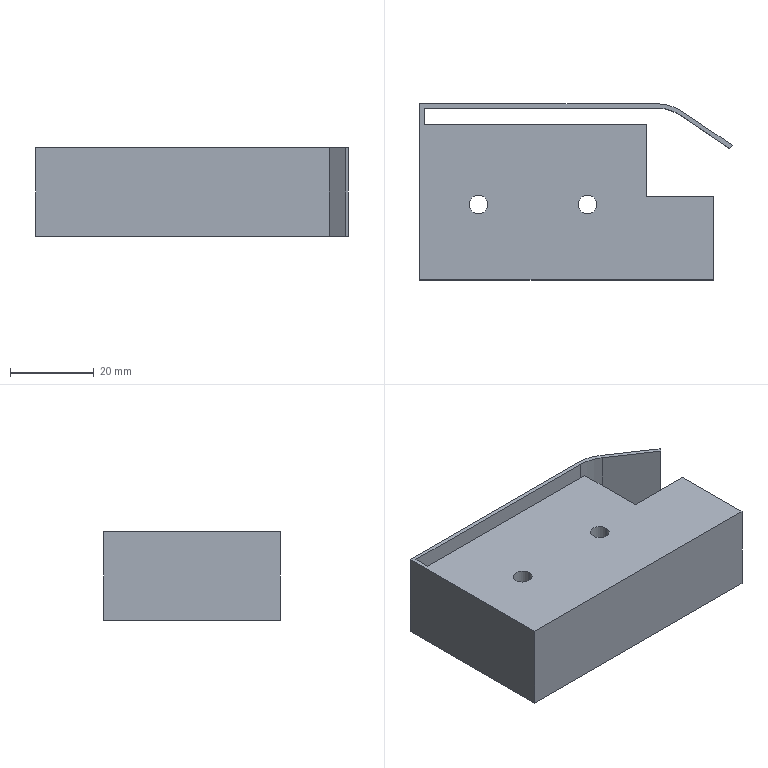Part | SolidWorks | features Extrusion 1, ICE 1 | 1 solid | 20 faces | box 74.506 x 42 x 21 mm | volume 49715 mm3 | plane 14 | cylinder 6 | commonest cylinder face diameters 4.5 x4 20 x2
STEP:
#1=CARTESIAN_POINT('',(37.75,18.,21.));
#2=VERTEX_POINT('',#1);
#3=CARTESIAN_POINT('',(42.25,18.,21.));
#4=VERTEX_POINT('',#3);
#5=CARTESIAN_POINT('',(40.,18.,21.));
#6=DIRECTION('',(0.,0.,1.));
#7=DIRECTION('',(1.,0.,0.));
#8=AXIS2_PLACEMENT_3D('',#5,#6,#7);
#9=CIRCLE('',#8,2.25);
#10=EDGE_CURVE('',#2,#4,#9,.T.);
#11=ORIENTED_EDGE('',*,*,#10,.T.);
#12=CARTESIAN_POINT('',(42.25,18.,0.));
#13=VERTEX_POINT('',#12);
#14=CARTESIAN_POINT('',(42.25,18.,21.));
#15=DIRECTION('',(0.,0.,-1.));
#16=VECTOR('',#15,1000.);
#17=LINE('',#14,#16);
#18=EDGE_CURVE('',#4,#13,#17,.T.);
#19=ORIENTED_EDGE('',*,*,#18,.T.);
#20=CARTESIAN_POINT('',(37.75,18.,0.));
#21=VERTEX_POINT('',#20);
#22=CARTESIAN_POINT('',(40.,18.,0.));
#23=DIRECTION('',(0.,0.,1.));
#24=DIRECTION('',(1.,0.,0.));
#25=AXIS2_PLACEMENT_3D('',#22,#23,#24);
#26=CIRCLE('',#25,2.25);
#27=EDGE_CURVE('',#21,#13,#26,.T.);
#28=ORIENTED_EDGE('',*,*,#27,.F.);
#29=CARTESIAN_POINT('',(37.75,18.,21.));
#30=DIRECTION('',(0.,0.,-1.));
#31=VECTOR('',#30,1000.);
#32=LINE('',#29,#31);
#33=EDGE_CURVE('',#2,#21,#32,.T.);
#34=ORIENTED_EDGE('',*,*,#33,.F.);
#35=EDGE_LOOP('',(#11,#19,#28,#34));
#36=FACE_OUTER_BOUND('',#35,.T.);
#37=CARTESIAN_POINT('',(40.,18.,21.));
#38=DIRECTION('',(0.,0.,-1.));
#39=DIRECTION('',(-1.,0.,0.));
#40=AXIS2_PLACEMENT_3D('',#37,#38,#39);
#41=CYLINDRICAL_SURFACE('',#40,2.25);
#42=ADVANCED_FACE('',(#36),#41,.F.);
#43=CARTESIAN_POINT('',(11.75,18.,21.));
#44=VERTEX_POINT('',#43);
#45=CARTESIAN_POINT('',(16.25,18.,21.));
#46=VERTEX_POINT('',#45);
#47=CARTESIAN_POINT('',(14.,18.,21.));
#48=DIRECTION('',(0.,0.,1.));
#49=DIRECTION('',(1.,0.,0.));
#50=AXIS2_PLACEMENT_3D('',#47,#48,#49);
#51=CIRCLE('',#50,2.25);
#52=EDGE_CURVE('',#44,#46,#51,.T.);
#53=ORIENTED_EDGE('',*,*,#52,.T.);
#54=CARTESIAN_POINT('',(16.25,18.,0.));
#55=VERTEX_POINT('',#54);
#56=CARTESIAN_POINT('',(16.25,18.,21.));
#57=DIRECTION('',(0.,0.,-1.));
#58=VECTOR('',#57,1000.);
#59=LINE('',#56,#58);
#60=EDGE_CURVE('',#46,#55,#59,.T.);
#61=ORIENTED_EDGE('',*,*,#60,.T.);
#62=CARTESIAN_POINT('',(11.75,18.,0.));
#63=VERTEX_POINT('',#62);
#64=CARTESIAN_POINT('',(14.,18.,0.));
#65=DIRECTION('',(0.,0.,1.));
#66=DIRECTION('',(1.,0.,0.));
#67=AXIS2_PLACEMENT_3D('',#64,#65,#66);
#68=CIRCLE('',#67,2.25);
#69=EDGE_CURVE('',#63,#55,#68,.T.);
#70=ORIENTED_EDGE('',*,*,#69,.F.);
#71=CARTESIAN_POINT('',(11.75,18.,21.));
#72=DIRECTION('',(0.,0.,-1.));
#73=VECTOR('',#72,1000.);
#74=LINE('',#71,#73);
#75=EDGE_CURVE('',#44,#63,#74,.T.);
#76=ORIENTED_EDGE('',*,*,#75,.F.);
#77=EDGE_LOOP('',(#53,#61,#70,#76));
#78=FACE_OUTER_BOUND('',#77,.T.);
#79=CARTESIAN_POINT('',(14.,18.,21.));
#80=DIRECTION('',(0.,0.,-1.));
#81=DIRECTION('',(-1.,0.,0.));
#82=AXIS2_PLACEMENT_3D('',#79,#80,#81);
#83=CYLINDRICAL_SURFACE('',#82,2.25);
#84=ADVANCED_FACE('',(#78),#83,.F.);
#85=ORIENTED_EDGE('',*,*,#52,.F.);
#86=CARTESIAN_POINT('',(14.,18.,21.));
#87=DIRECTION('',(0.,0.,1.));
#88=DIRECTION('',(1.,0.,0.));
#89=AXIS2_PLACEMENT_3D('',#86,#87,#88);
#90=CIRCLE('',#89,2.25);
#91=EDGE_CURVE('',#46,#44,#90,.T.);
#92=ORIENTED_EDGE('',*,*,#91,.F.);
#93=EDGE_LOOP('',(#85,#92));
#94=FACE_BOUND('',#93,.T.);
#95=CARTESIAN_POINT('',(0.,42.,21.));
#96=VERTEX_POINT('',#95);
#97=CARTESIAN_POINT('',(0.,0.,21.));
#98=VERTEX_POINT('',#97);
#99=CARTESIAN_POINT('',(0.,0.,21.));
#100=DIRECTION('',(0.,-1.,0.));
#101=VECTOR('',#100,1000.);
#102=LINE('',#99,#101);
#103=EDGE_CURVE('',#96,#98,#102,.T.);
#104=ORIENTED_EDGE('',*,*,#103,.T.);
#105=CARTESIAN_POINT('',(70.,0.,21.));
#106=VERTEX_POINT('',#105);
#107=CARTESIAN_POINT('',(0.,0.,21.));
#108=DIRECTION('',(1.,0.,0.));
#109=VECTOR('',#108,1000.);
#110=LINE('',#107,#109);
#111=EDGE_CURVE('',#98,#106,#110,.T.);
#112=ORIENTED_EDGE('',*,*,#111,.T.);
#113=CARTESIAN_POINT('',(70.,20.,21.));
#114=VERTEX_POINT('',#113);
#115=CARTESIAN_POINT('',(70.,0.,21.));
#116=DIRECTION('',(0.,1.,0.));
#117=VECTOR('',#116,1000.);
#118=LINE('',#115,#117);
#119=EDGE_CURVE('',#106,#114,#118,.T.);
#120=ORIENTED_EDGE('',*,*,#119,.T.);
#121=CARTESIAN_POINT('',(54.,20.,21.));
#122=VERTEX_POINT('',#121);
#123=CARTESIAN_POINT('',(54.,20.,21.));
#124=DIRECTION('',(-1.,0.,0.));
#125=VECTOR('',#124,1000.);
#126=LINE('',#123,#125);
#127=EDGE_CURVE('',#114,#122,#126,.T.);
#128=ORIENTED_EDGE('',*,*,#127,.T.);
#129=CARTESIAN_POINT('',(54.,37.,21.));
#130=VERTEX_POINT('',#129);
#131=CARTESIAN_POINT('',(54.,20.,21.));
#132=DIRECTION('',(0.,1.,0.));
#133=VECTOR('',#132,1000.);
#134=LINE('',#131,#133);
#135=EDGE_CURVE('',#122,#130,#134,.T.);
#136=ORIENTED_EDGE('',*,*,#135,.T.);
#137=CARTESIAN_POINT('',(1.,37.,21.));
#138=VERTEX_POINT('',#137);
#139=CARTESIAN_POINT('',(0.,37.,21.));
#140=DIRECTION('',(-1.,0.,0.));
#141=VECTOR('',#140,1000.);
#142=LINE('',#139,#141);
#143=EDGE_CURVE('',#130,#138,#142,.T.);
#144=ORIENTED_EDGE('',*,*,#143,.T.);
#145=CARTESIAN_POINT('',(1.,41.,21.));
#146=VERTEX_POINT('',#145);
#147=CARTESIAN_POINT('',(1.,37.,21.));
#148=DIRECTION('',(0.,1.,0.));
#149=VECTOR('',#148,1000.);
#150=LINE('',#147,#149);
#151=EDGE_CURVE('',#138,#146,#150,.T.);
#152=ORIENTED_EDGE('',*,*,#151,.T.);
#153=CARTESIAN_POINT('',(56.534,41.,21.));
#154=VERTEX_POINT('',#153);
#155=CARTESIAN_POINT('',(1.,41.,21.));
#156=DIRECTION('',(1.,0.,0.));
#157=VECTOR('',#156,1000.);
#158=LINE('',#155,#157);
#159=EDGE_CURVE('',#146,#154,#158,.T.);
#160=ORIENTED_EDGE('',*,*,#159,.T.);
#161=CARTESIAN_POINT('',(62.118,39.295,21.));
#162=VERTEX_POINT('',#161);
#163=CARTESIAN_POINT('',(56.534,31.,21.));
#164=DIRECTION('',(0.,0.,-1.));
#165=DIRECTION('',(1.,0.,0.));
#166=AXIS2_PLACEMENT_3D('',#163,#164,#165);
#167=CIRCLE('',#166,10.);
#168=EDGE_CURVE('',#154,#162,#167,.T.);
#169=ORIENTED_EDGE('',*,*,#168,.T.);
#170=CARTESIAN_POINT('',(73.948,31.331,21.));
#171=VERTEX_POINT('',#170);
#172=CARTESIAN_POINT('',(62.118,39.295,21.));
#173=DIRECTION('',(0.8295,-0.5585,0.));
#174=VECTOR('',#173,1000.);
#175=LINE('',#172,#174);
#176=EDGE_CURVE('',#162,#171,#175,.T.);
#177=ORIENTED_EDGE('',*,*,#176,.T.);
#178=CARTESIAN_POINT('',(74.506,32.16,21.));
#179=VERTEX_POINT('',#178);
#180=CARTESIAN_POINT('',(74.506,32.16,21.));
#181=DIRECTION('',(0.5585,0.8295,0.));
#182=VECTOR('',#181,1000.);
#183=LINE('',#180,#182);
#184=EDGE_CURVE('',#171,#179,#183,.T.);
#185=ORIENTED_EDGE('',*,*,#184,.T.);
#186=CARTESIAN_POINT('',(62.424,40.295,21.));
#187=VERTEX_POINT('',#186);
#188=CARTESIAN_POINT('',(62.424,40.295,21.));
#189=DIRECTION('',(-0.8295,0.5585,0.));
#190=VECTOR('',#189,1000.);
#191=LINE('',#188,#190);
#192=EDGE_CURVE('',#179,#187,#191,.T.);
#193=ORIENTED_EDGE('',*,*,#192,.T.);
#194=CARTESIAN_POINT('',(56.839,42.,21.));
#195=VERTEX_POINT('',#194);
#196=CARTESIAN_POINT('',(56.839,32.,21.));
#197=DIRECTION('',(0.,0.,1.));
#198=DIRECTION('',(1.,0.,0.));
#199=AXIS2_PLACEMENT_3D('',#196,#197,#198);
#200=CIRCLE('',#199,10.);
#201=EDGE_CURVE('',#187,#195,#200,.T.);
#202=ORIENTED_EDGE('',*,*,#201,.T.);
#203=CARTESIAN_POINT('',(0.,42.,21.));
#204=DIRECTION('',(-1.,0.,0.));
#205=VECTOR('',#204,1000.);
#206=LINE('',#203,#205);
#207=EDGE_CURVE('',#195,#96,#206,.T.);
#208=ORIENTED_EDGE('',*,*,#207,.T.);
#209=EDGE_LOOP('',(#104,#112,#120,#128,#136,#144,#152,#160,#169,#177,#185,#193,#202,#208));
#210=FACE_OUTER_BOUND('',#209,.T.);
#211=ORIENTED_EDGE('',*,*,#10,.F.);
#212=CARTESIAN_POINT('',(40.,18.,21.));
#213=DIRECTION('',(0.,0.,1.));
#214=DIRECTION('',(1.,0.,0.));
#215=AXIS2_PLACEMENT_3D('',#212,#213,#214);
#216=CIRCLE('',#215,2.25);
#217=EDGE_CURVE('',#4,#2,#216,.T.);
#218=ORIENTED_EDGE('',*,*,#217,.F.);
#219=EDGE_LOOP('',(#211,#218));
#220=FACE_BOUND('',#219,.T.);
#221=CARTESIAN_POINT('',(0.,37.,21.));
#222=DIRECTION('',(0.,0.,-1.));
#223=DIRECTION('',(-1.,0.,0.));
#224=AXIS2_PLACEMENT_3D('',#221,#222,#223);
#225=PLANE('',#224);
#226=ADVANCED_FACE('',(#94,#210,#220),#225,.F.);
#227=ORIENTED_EDGE('',*,*,#69,.T.);
#228=CARTESIAN_POINT('',(14.,18.,0.));
#229=DIRECTION('',(0.,0.,1.));
#230=DIRECTION('',(1.,0.,0.));
#231=AXIS2_PLACEMENT_3D('',#228,#229,#230);
#232=CIRCLE('',#231,2.25);
#233=EDGE_CURVE('',#55,#63,#232,.T.);
#234=ORIENTED_EDGE('',*,*,#233,.T.);
#235=EDGE_LOOP('',(#227,#234));
#236=FACE_BOUND('',#235,.T.);
#237=CARTESIAN_POINT('',(0.,42.,0.));
#238=VERTEX_POINT('',#237);
#239=CARTESIAN_POINT('',(0.,0.,0.));
#240=VERTEX_POINT('',#239);
#241=CARTESIAN_POINT('',(0.,0.,0.));
#242=DIRECTION('',(0.,-1.,0.));
#243=VECTOR('',#242,1000.);
#244=LINE('',#241,#243);
#245=EDGE_CURVE('',#238,#240,#244,.T.);
#246=ORIENTED_EDGE('',*,*,#245,.F.);
#247=CARTESIAN_POINT('',(56.839,42.,0.));
#248=VERTEX_POINT('',#247);
#249=CARTESIAN_POINT('',(0.,42.,0.));
#250=DIRECTION('',(-1.,0.,0.));
#251=VECTOR('',#250,1000.);
#252=LINE('',#249,#251);
#253=EDGE_CURVE('',#248,#238,#252,.T.);
#254=ORIENTED_EDGE('',*,*,#253,.F.);
#255=CARTESIAN_POINT('',(62.424,40.295,0.));
#256=VERTEX_POINT('',#255);
#257=CARTESIAN_POINT('',(56.839,32.,0.));
#258=DIRECTION('',(0.,0.,1.));
#259=DIRECTION('',(-1.,0.,0.));
#260=AXIS2_PLACEMENT_3D('',#257,#258,#259);
#261=CIRCLE('',#260,10.);
#262=EDGE_CURVE('',#256,#248,#261,.T.);
#263=ORIENTED_EDGE('',*,*,#262,.F.);
#264=CARTESIAN_POINT('',(74.506,32.16,0.));
#265=VERTEX_POINT('',#264);
#266=CARTESIAN_POINT('',(62.424,40.295,0.));
#267=DIRECTION('',(-0.8295,0.5585,0.));
#268=VECTOR('',#267,1000.);
#269=LINE('',#266,#268);
#270=EDGE_CURVE('',#265,#256,#269,.T.);
#271=ORIENTED_EDGE('',*,*,#270,.F.);
#272=CARTESIAN_POINT('',(73.948,31.331,0.));
#273=VERTEX_POINT('',#272);
#274=CARTESIAN_POINT('',(74.506,32.16,0.));
#275=DIRECTION('',(0.5585,0.8295,0.));
#276=VECTOR('',#275,1000.);
#277=LINE('',#274,#276);
#278=EDGE_CURVE('',#273,#265,#277,.T.);
#279=ORIENTED_EDGE('',*,*,#278,.F.);
#280=CARTESIAN_POINT('',(62.118,39.295,0.));
#281=VERTEX_POINT('',#280);
#282=CARTESIAN_POINT('',(62.118,39.295,0.));
#283=DIRECTION('',(0.8295,-0.5585,0.));
#284=VECTOR('',#283,1000.);
#285=LINE('',#282,#284);
#286=EDGE_CURVE('',#281,#273,#285,.T.);
#287=ORIENTED_EDGE('',*,*,#286,.F.);
#288=CARTESIAN_POINT('',(56.534,41.,0.));
#289=VERTEX_POINT('',#288);
#290=CARTESIAN_POINT('',(56.534,31.,0.));
#291=DIRECTION('',(0.,0.,-1.));
#292=DIRECTION('',(-1.,0.,0.));
#293=AXIS2_PLACEMENT_3D('',#290,#291,#292);
#294=CIRCLE('',#293,10.);
#295=EDGE_CURVE('',#289,#281,#294,.T.);
#296=ORIENTED_EDGE('',*,*,#295,.F.);
#297=CARTESIAN_POINT('',(1.,41.,0.));
#298=VERTEX_POINT('',#297);
#299=CARTESIAN_POINT('',(1.,41.,0.));
#300=DIRECTION('',(1.,0.,0.));
#301=VECTOR('',#300,1000.);
#302=LINE('',#299,#301);
#303=EDGE_CURVE('',#298,#289,#302,.T.);
#304=ORIENTED_EDGE('',*,*,#303,.F.);
#305=CARTESIAN_POINT('',(1.,37.,0.));
#306=VERTEX_POINT('',#305);
#307=CARTESIAN_POINT('',(1.,37.,0.));
#308=DIRECTION('',(0.,1.,0.));
#309=VECTOR('',#308,1000.);
#310=LINE('',#307,#309);
#311=EDGE_CURVE('',#306,#298,#310,.T.);
#312=ORIENTED_EDGE('',*,*,#311,.F.);
#313=CARTESIAN_POINT('',(54.,37.,0.));
#314=VERTEX_POINT('',#313);
#315=CARTESIAN_POINT('',(0.,37.,0.));
#316=DIRECTION('',(-1.,0.,0.));
#317=VECTOR('',#316,1000.);
#318=LINE('',#315,#317);
#319=EDGE_CURVE('',#314,#306,#318,.T.);
#320=ORIENTED_EDGE('',*,*,#319,.F.);
#321=CARTESIAN_POINT('',(54.,20.,0.));
#322=VERTEX_POINT('',#321);
#323=CARTESIAN_POINT('',(54.,20.,0.));
#324=DIRECTION('',(0.,1.,0.));
#325=VECTOR('',#324,1000.);
#326=LINE('',#323,#325);
#327=EDGE_CURVE('',#322,#314,#326,.T.);
#328=ORIENTED_EDGE('',*,*,#327,.F.);
#329=CARTESIAN_POINT('',(70.,20.,0.));
#330=VERTEX_POINT('',#329);
#331=CARTESIAN_POINT('',(54.,20.,0.));
#332=DIRECTION('',(-1.,0.,0.));
#333=VECTOR('',#332,1000.);
#334=LINE('',#331,#333);
#335=EDGE_CURVE('',#330,#322,#334,.T.);
#336=ORIENTED_EDGE('',*,*,#335,.F.);
#337=CARTESIAN_POINT('',(70.,0.,0.));
#338=VERTEX_POINT('',#337);
#339=CARTESIAN_POINT('',(70.,0.,0.));
#340=DIRECTION('',(0.,1.,0.));
#341=VECTOR('',#340,1000.);
#342=LINE('',#339,#341);
#343=EDGE_CURVE('',#338,#330,#342,.T.);
#344=ORIENTED_EDGE('',*,*,#343,.F.);
#345=CARTESIAN_POINT('',(0.,0.,0.));
#346=DIRECTION('',(1.,0.,0.));
#347=VECTOR('',#346,1000.);
#348=LINE('',#345,#347);
#349=EDGE_CURVE('',#240,#338,#348,.T.);
#350=ORIENTED_EDGE('',*,*,#349,.F.);
#351=EDGE_LOOP('',(#246,#254,#263,#271,#279,#287,#296,#304,#312,#320,#328,#336,#344,#350));
#352=FACE_OUTER_BOUND('',#351,.T.);
#353=ORIENTED_EDGE('',*,*,#27,.T.);
#354=CARTESIAN_POINT('',(40.,18.,0.));
#355=DIRECTION('',(0.,0.,1.));
#356=DIRECTION('',(1.,0.,0.));
#357=AXIS2_PLACEMENT_3D('',#354,#355,#356);
#358=CIRCLE('',#357,2.25);
#359=EDGE_CURVE('',#13,#21,#358,.T.);
#360=ORIENTED_EDGE('',*,*,#359,.T.);
#361=EDGE_LOOP('',(#353,#360));
#362=FACE_BOUND('',#361,.T.);
#363=CARTESIAN_POINT('',(0.,37.,0.));
#364=DIRECTION('',(0.,0.,-1.));
#365=DIRECTION('',(-1.,0.,0.));
#366=AXIS2_PLACEMENT_3D('',#363,#364,#365);
#367=PLANE('',#366);
#368=ADVANCED_FACE('',(#236,#352,#362),#367,.T.);
#369=ORIENTED_EDGE('',*,*,#245,.T.);
#370=CARTESIAN_POINT('',(0.,0.,21.));
#371=DIRECTION('',(0.,0.,-1.));
#372=VECTOR('',#371,1000.);
#373=LINE('',#370,#372);
#374=EDGE_CURVE('',#98,#240,#373,.T.);
#375=ORIENTED_EDGE('',*,*,#374,.F.);
#376=ORIENTED_EDGE('',*,*,#103,.F.);
#377=CARTESIAN_POINT('',(0.,42.,-75.266));
#378=DIRECTION('',(0.,0.,1.));
#379=VECTOR('',#378,1000.);
#380=LINE('',#377,#379);
#381=EDGE_CURVE('',#238,#96,#380,.T.);
#382=ORIENTED_EDGE('',*,*,#381,.F.);
#383=EDGE_LOOP('',(#369,#375,#376,#382));
#384=FACE_OUTER_BOUND('',#383,.T.);
#385=CARTESIAN_POINT('',(0.,0.,21.));
#386=DIRECTION('',(1.,0.,0.));
#387=DIRECTION('',(0.,0.,-1.));
#388=AXIS2_PLACEMENT_3D('',#385,#386,#387);
#389=PLANE('',#388);
#390=ADVANCED_FACE('',(#384),#389,.F.);
#391=ORIENTED_EDGE('',*,*,#349,.T.);
#392=CARTESIAN_POINT('',(70.,0.,21.));
#393=DIRECTION('',(0.,0.,-1.));
#394=VECTOR('',#393,1000.);
#395=LINE('',#392,#394);
#396=EDGE_CURVE('',#106,#338,#395,.T.);
#397=ORIENTED_EDGE('',*,*,#396,.F.);
#398=ORIENTED_EDGE('',*,*,#111,.F.);
#399=ORIENTED_EDGE('',*,*,#374,.T.);
#400=EDGE_LOOP('',(#391,#397,#398,#399));
#401=FACE_OUTER_BOUND('',#400,.T.);
#402=CARTESIAN_POINT('',(0.,0.,21.));
#403=DIRECTION('',(0.,1.,0.));
#404=DIRECTION('',(0.,0.,1.));
#405=AXIS2_PLACEMENT_3D('',#402,#403,#404);
#406=PLANE('',#405);
#407=ADVANCED_FACE('',(#401),#406,.F.);
#408=ORIENTED_EDGE('',*,*,#343,.T.);
#409=CARTESIAN_POINT('',(70.,20.,21.));
#410=DIRECTION('',(0.,0.,-1.));
#411=VECTOR('',#410,1000.);
#412=LINE('',#409,#411);
#413=EDGE_CURVE('',#114,#330,#412,.T.);
#414=ORIENTED_EDGE('',*,*,#413,.F.);
#415=ORIENTED_EDGE('',*,*,#119,.F.);
#416=ORIENTED_EDGE('',*,*,#396,.T.);
#417=EDGE_LOOP('',(#408,#414,#415,#416));
#418=FACE_OUTER_BOUND('',#417,.T.);
#419=CARTESIAN_POINT('',(70.,0.,21.));
#420=DIRECTION('',(-1.,0.,0.));
#421=DIRECTION('',(0.,0.,1.));
#422=AXIS2_PLACEMENT_3D('',#419,#420,#421);
#423=PLANE('',#422);
#424=ADVANCED_FACE('',(#418),#423,.F.);
#425=ORIENTED_EDGE('',*,*,#335,.T.);
#426=CARTESIAN_POINT('',(54.,20.,21.));
#427=DIRECTION('',(0.,0.,-1.));
#428=VECTOR('',#427,1000.);
#429=LINE('',#426,#428);
#430=EDGE_CURVE('',#122,#322,#429,.T.);
#431=ORIENTED_EDGE('',*,*,#430,.F.);
#432=ORIENTED_EDGE('',*,*,#127,.F.);
#433=ORIENTED_EDGE('',*,*,#413,.T.);
#434=EDGE_LOOP('',(#425,#431,#432,#433));
#435=FACE_OUTER_BOUND('',#434,.T.);
#436=CARTESIAN_POINT('',(54.,20.,21.));
#437=DIRECTION('',(0.,-1.,0.));
#438=DIRECTION('',(0.,0.,-1.));
#439=AXIS2_PLACEMENT_3D('',#436,#437,#438);
#440=PLANE('',#439);
#441=ADVANCED_FACE('',(#435),#440,.F.);
#442=ORIENTED_EDGE('',*,*,#327,.T.);
#443=CARTESIAN_POINT('',(54.,37.,21.));
#444=DIRECTION('',(0.,0.,-1.));
#445=VECTOR('',#444,1000.);
#446=LINE('',#443,#445);
#447=EDGE_CURVE('',#130,#314,#446,.T.);
#448=ORIENTED_EDGE('',*,*,#447,.F.);
#449=ORIENTED_EDGE('',*,*,#135,.F.);
#450=ORIENTED_EDGE('',*,*,#430,.T.);
#451=EDGE_LOOP('',(#442,#448,#449,#450));
#452=FACE_OUTER_BOUND('',#451,.T.);
#453=CARTESIAN_POINT('',(54.,20.,21.));
#454=DIRECTION('',(-1.,0.,0.));
#455=DIRECTION('',(0.,0.,1.));
#456=AXIS2_PLACEMENT_3D('',#453,#454,#455);
#457=PLANE('',#456);
#458=ADVANCED_FACE('',(#452),#457,.F.);
#459=ORIENTED_EDGE('',*,*,#319,.T.);
#460=CARTESIAN_POINT('',(1.,37.,-75.266));
#461=DIRECTION('',(0.,0.,1.));
#462=VECTOR('',#461,1000.);
#463=LINE('',#460,#462);
#464=EDGE_CURVE('',#306,#138,#463,.T.);
#465=ORIENTED_EDGE('',*,*,#464,.T.);
#466=ORIENTED_EDGE('',*,*,#143,.F.);
#467=ORIENTED_EDGE('',*,*,#447,.T.);
#468=EDGE_LOOP('',(#459,#465,#466,#467));
#469=FACE_OUTER_BOUND('',#468,.T.);
#470=CARTESIAN_POINT('',(0.,37.,21.));
#471=DIRECTION('',(0.,-1.,0.));
#472=DIRECTION('',(0.,0.,-1.));
#473=AXIS2_PLACEMENT_3D('',#470,#471,#472);
#474=PLANE('',#473);
#475=ADVANCED_FACE('',(#469),#474,.F.);
#476=ORIENTED_EDGE('',*,*,#60,.F.);
#477=ORIENTED_EDGE('',*,*,#91,.T.);
#478=ORIENTED_EDGE('',*,*,#75,.T.);
#479=ORIENTED_EDGE('',*,*,#233,.F.);
#480=EDGE_LOOP('',(#476,#477,#478,#479));
#481=FACE_OUTER_BOUND('',#480,.T.);
#482=CARTESIAN_POINT('',(14.,18.,21.));
#483=DIRECTION('',(0.,0.,-1.));
#484=DIRECTION('',(-1.,0.,0.));
#485=AXIS2_PLACEMENT_3D('',#482,#483,#484);
#486=CYLINDRICAL_SURFACE('',#485,2.25);
#487=ADVANCED_FACE('',(#481),#486,.F.);
#488=ORIENTED_EDGE('',*,*,#18,.F.);
#489=ORIENTED_EDGE('',*,*,#217,.T.);
#490=ORIENTED_EDGE('',*,*,#33,.T.);
#491=ORIENTED_EDGE('',*,*,#359,.F.);
#492=EDGE_LOOP('',(#488,#489,#490,#491));
#493=FACE_OUTER_BOUND('',#492,.T.);
#494=CARTESIAN_POINT('',(40.,18.,21.));
#495=DIRECTION('',(0.,0.,-1.));
#496=DIRECTION('',(-1.,0.,0.));
#497=AXIS2_PLACEMENT_3D('',#494,#495,#496);
#498=CYLINDRICAL_SURFACE('',#497,2.25);
#499=ADVANCED_FACE('',(#493),#498,.F.);
#500=ORIENTED_EDGE('',*,*,#464,.F.);
#501=ORIENTED_EDGE('',*,*,#311,.T.);
#502=CARTESIAN_POINT('',(1.,41.,-75.266));
#503=DIRECTION('',(0.,0.,1.));
#504=VECTOR('',#503,1000.);
#505=LINE('',#502,#504);
#506=EDGE_CURVE('',#298,#146,#505,.T.);
#507=ORIENTED_EDGE('',*,*,#506,.T.);
#508=ORIENTED_EDGE('',*,*,#151,.F.);
#509=EDGE_LOOP('',(#500,#501,#507,#508));
#510=FACE_OUTER_BOUND('',#509,.T.);
#511=CARTESIAN_POINT('',(1.,37.,-75.266));
#512=DIRECTION('',(1.,0.,0.));
#513=DIRECTION('',(0.,0.,-1.));
#514=AXIS2_PLACEMENT_3D('',#511,#512,#513);
#515=PLANE('',#514);
#516=ADVANCED_FACE('',(#510),#515,.T.);
#517=ORIENTED_EDGE('',*,*,#506,.F.);
#518=ORIENTED_EDGE('',*,*,#303,.T.);
#519=CARTESIAN_POINT('',(56.534,41.,-75.266));
#520=DIRECTION('',(0.,0.,1.));
#521=VECTOR('',#520,1000.);
#522=LINE('',#519,#521);
#523=EDGE_CURVE('',#289,#154,#522,.T.);
#524=ORIENTED_EDGE('',*,*,#523,.T.);
#525=ORIENTED_EDGE('',*,*,#159,.F.);
#526=EDGE_LOOP('',(#517,#518,#524,#525));
#527=FACE_OUTER_BOUND('',#526,.T.);
#528=CARTESIAN_POINT('',(1.,41.,-75.266));
#529=DIRECTION('',(0.,-1.,0.));
#530=DIRECTION('',(0.,0.,-1.));
#531=AXIS2_PLACEMENT_3D('',#528,#529,#530);
#532=PLANE('',#531);
#533=ADVANCED_FACE('',(#527),#532,.T.);
#534=ORIENTED_EDGE('',*,*,#523,.F.);
#535=ORIENTED_EDGE('',*,*,#295,.T.);
#536=CARTESIAN_POINT('',(62.118,39.295,-75.266));
#537=DIRECTION('',(0.,0.,1.));
#538=VECTOR('',#537,1000.);
#539=LINE('',#536,#538);
#540=EDGE_CURVE('',#281,#162,#539,.T.);
#541=ORIENTED_EDGE('',*,*,#540,.T.);
#542=ORIENTED_EDGE('',*,*,#168,.F.);
#543=EDGE_LOOP('',(#534,#535,#541,#542));
#544=FACE_OUTER_BOUND('',#543,.T.);
#545=CARTESIAN_POINT('',(56.534,31.,-75.266));
#546=DIRECTION('',(0.,0.,1.));
#547=DIRECTION('',(1.,0.,0.));
#548=AXIS2_PLACEMENT_3D('',#545,#546,#547);
#549=CYLINDRICAL_SURFACE('',#548,10.);
#550=ADVANCED_FACE('',(#544),#549,.F.);
#551=ORIENTED_EDGE('',*,*,#540,.F.);
#552=ORIENTED_EDGE('',*,*,#286,.T.);
#553=CARTESIAN_POINT('',(73.948,31.331,-75.266));
#554=DIRECTION('',(0.,0.,1.));
#555=VECTOR('',#554,1000.);
#556=LINE('',#553,#555);
#557=EDGE_CURVE('',#273,#171,#556,.T.);
#558=ORIENTED_EDGE('',*,*,#557,.T.);
#559=ORIENTED_EDGE('',*,*,#176,.F.);
#560=EDGE_LOOP('',(#551,#552,#558,#559));
#561=FACE_OUTER_BOUND('',#560,.T.);
#562=CARTESIAN_POINT('',(62.118,39.295,-75.266));
#563=DIRECTION('',(-0.5585,-0.8295,0.));
#564=DIRECTION('',(0.8295,-0.5585,0.));
#565=AXIS2_PLACEMENT_3D('',#562,#563,#564);
#566=PLANE('',#565);
#567=ADVANCED_FACE('',(#561),#566,.T.);
#568=ORIENTED_EDGE('',*,*,#557,.F.);
#569=ORIENTED_EDGE('',*,*,#278,.T.);
#570=CARTESIAN_POINT('',(74.506,32.16,-75.266));
#571=DIRECTION('',(0.,0.,1.));
#572=VECTOR('',#571,1000.);
#573=LINE('',#570,#572);
#574=EDGE_CURVE('',#265,#179,#573,.T.);
#575=ORIENTED_EDGE('',*,*,#574,.T.);
#576=ORIENTED_EDGE('',*,*,#184,.F.);
#577=EDGE_LOOP('',(#568,#569,#575,#576));
#578=FACE_OUTER_BOUND('',#577,.T.);
#579=CARTESIAN_POINT('',(74.506,32.16,-75.266));
#580=DIRECTION('',(0.8295,-0.5585,0.));
#581=DIRECTION('',(0.5585,0.8295,0.));
#582=AXIS2_PLACEMENT_3D('',#579,#580,#581);
#583=PLANE('',#582);
#584=ADVANCED_FACE('',(#578),#583,.T.);
#585=ORIENTED_EDGE('',*,*,#574,.F.);
#586=ORIENTED_EDGE('',*,*,#270,.T.);
#587=CARTESIAN_POINT('',(62.424,40.295,-75.266));
#588=DIRECTION('',(0.,0.,1.));
#589=VECTOR('',#588,1000.);
#590=LINE('',#587,#589);
#591=EDGE_CURVE('',#256,#187,#590,.T.);
#592=ORIENTED_EDGE('',*,*,#591,.T.);
#593=ORIENTED_EDGE('',*,*,#192,.F.);
#594=EDGE_LOOP('',(#585,#586,#592,#593));
#595=FACE_OUTER_BOUND('',#594,.T.);
#596=CARTESIAN_POINT('',(62.424,40.295,-75.266));
#597=DIRECTION('',(0.5585,0.8295,0.));
#598=DIRECTION('',(-0.8295,0.5585,0.));
#599=AXIS2_PLACEMENT_3D('',#596,#597,#598);
#600=PLANE('',#599);
#601=ADVANCED_FACE('',(#595),#600,.T.);
#602=ORIENTED_EDGE('',*,*,#591,.F.);
#603=ORIENTED_EDGE('',*,*,#262,.T.);
#604=CARTESIAN_POINT('',(56.839,42.,-75.266));
#605=DIRECTION('',(0.,0.,1.));
#606=VECTOR('',#605,1000.);
#607=LINE('',#604,#606);
#608=EDGE_CURVE('',#248,#195,#607,.T.);
#609=ORIENTED_EDGE('',*,*,#608,.T.);
#610=ORIENTED_EDGE('',*,*,#201,.F.);
#611=EDGE_LOOP('',(#602,#603,#609,#610));
#612=FACE_OUTER_BOUND('',#611,.T.);
#613=CARTESIAN_POINT('',(56.839,32.,-75.266));
#614=DIRECTION('',(0.,0.,1.));
#615=DIRECTION('',(1.,0.,0.));
#616=AXIS2_PLACEMENT_3D('',#613,#614,#615);
#617=CYLINDRICAL_SURFACE('',#616,10.);
#618=ADVANCED_FACE('',(#612),#617,.T.);
#619=ORIENTED_EDGE('',*,*,#608,.F.);
#620=ORIENTED_EDGE('',*,*,#253,.T.);
#621=ORIENTED_EDGE('',*,*,#381,.T.);
#622=ORIENTED_EDGE('',*,*,#207,.F.);
#623=EDGE_LOOP('',(#619,#620,#621,#622));
#624=FACE_OUTER_BOUND('',#623,.T.);
#625=CARTESIAN_POINT('',(0.,42.,-75.266));
#626=DIRECTION('',(0.,1.,0.));
#627=DIRECTION('',(0.,0.,1.));
#628=AXIS2_PLACEMENT_3D('',#625,#626,#627);
#629=PLANE('',#628);
#630=ADVANCED_FACE('',(#624),#629,.T.);
#631=CLOSED_SHELL('',(#42,#84,#226,#368,#390,#407,#424,#441,#458,#475,#487,#499,#516,#533,#550,#567,#584,#601,#618,#630));
#632=MANIFOLD_SOLID_BREP('',#631);
#633=CARTESIAN_POINT('',(0.,0.,0.));
#634=DIRECTION('',(0.,0.,1.));
#635=DIRECTION('',(1.,0.,0.));
#636=AXIS2_PLACEMENT_3D('',#633,#634,#635);
#637=(LENGTH_UNIT()NAMED_UNIT(*)SI_UNIT(.MILLI.,.METRE.));
#638=UNCERTAINTY_MEASURE_WITH_UNIT(LENGTH_MEASURE(0.00001),#637,'','');
#639=(NAMED_UNIT(*)PLANE_ANGLE_UNIT()SI_UNIT($,.RADIAN.));
#640=(NAMED_UNIT(*)SI_UNIT($,.STERADIAN.)SOLID_ANGLE_UNIT());
#641=(GEOMETRIC_REPRESENTATION_CONTEXT(3)GLOBAL_UNCERTAINTY_ASSIGNED_CONTEXT((#638))GLOBAL_UNIT_ASSIGNED_CONTEXT((#637,#639,#640))REPRESENTATION_CONTEXT('',''));
#642=ADVANCED_BREP_SHAPE_REPRESENTATION('',(#632,#636),#641);